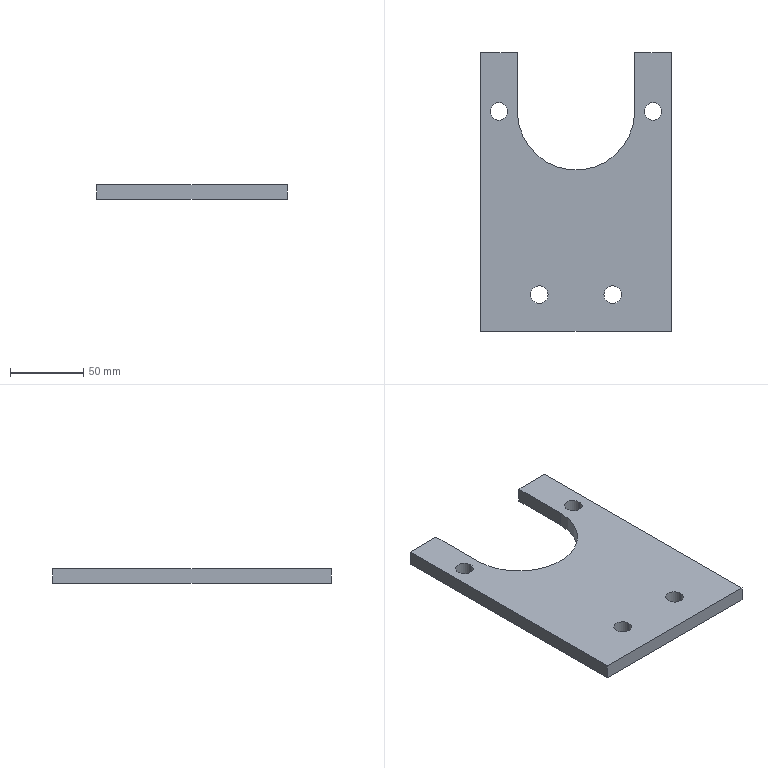Part | SolidWorks | features Extrusion 1 | 1 solid | 18 faces | box 130 x 190 x 10 mm | volume 185343 mm3 | cylinder 9 | plane 9 | commonest cylinder face diameters 12 x8 80 x1
STEP:
#1=CARTESIAN_POINT('',(84.,25.,10.));
#2=VERTEX_POINT('',#1);
#3=CARTESIAN_POINT('',(96.,25.,10.));
#4=VERTEX_POINT('',#3);
#5=CARTESIAN_POINT('',(90.,25.,10.));
#6=DIRECTION('',(0.,0.,1.));
#7=DIRECTION('',(1.,0.,0.));
#8=AXIS2_PLACEMENT_3D('',#5,#6,#7);
#9=CIRCLE('',#8,6.);
#10=EDGE_CURVE('',#2,#4,#9,.T.);
#11=ORIENTED_EDGE('',*,*,#10,.T.);
#12=CARTESIAN_POINT('',(96.,25.,0.));
#13=VERTEX_POINT('',#12);
#14=CARTESIAN_POINT('',(96.,25.,10.));
#15=DIRECTION('',(0.,0.,-1.));
#16=VECTOR('',#15,1000.);
#17=LINE('',#14,#16);
#18=EDGE_CURVE('',#4,#13,#17,.T.);
#19=ORIENTED_EDGE('',*,*,#18,.T.);
#20=CARTESIAN_POINT('',(84.,25.,0.));
#21=VERTEX_POINT('',#20);
#22=CARTESIAN_POINT('',(90.,25.,0.));
#23=DIRECTION('',(0.,0.,1.));
#24=DIRECTION('',(1.,0.,0.));
#25=AXIS2_PLACEMENT_3D('',#22,#23,#24);
#26=CIRCLE('',#25,6.);
#27=EDGE_CURVE('',#21,#13,#26,.T.);
#28=ORIENTED_EDGE('',*,*,#27,.F.);
#29=CARTESIAN_POINT('',(84.,25.,10.));
#30=DIRECTION('',(0.,0.,-1.));
#31=VECTOR('',#30,1000.);
#32=LINE('',#29,#31);
#33=EDGE_CURVE('',#2,#21,#32,.T.);
#34=ORIENTED_EDGE('',*,*,#33,.F.);
#35=EDGE_LOOP('',(#11,#19,#28,#34));
#36=FACE_OUTER_BOUND('',#35,.T.);
#37=CARTESIAN_POINT('',(90.,25.,10.));
#38=DIRECTION('',(0.,0.,-1.));
#39=DIRECTION('',(-1.,0.,0.));
#40=AXIS2_PLACEMENT_3D('',#37,#38,#39);
#41=CYLINDRICAL_SURFACE('',#40,6.);
#42=ADVANCED_FACE('',(#36),#41,.F.);
#43=CARTESIAN_POINT('',(34.,25.,10.));
#44=VERTEX_POINT('',#43);
#45=CARTESIAN_POINT('',(46.,25.,10.));
#46=VERTEX_POINT('',#45);
#47=CARTESIAN_POINT('',(40.,25.,10.));
#48=DIRECTION('',(0.,0.,1.));
#49=DIRECTION('',(1.,0.,0.));
#50=AXIS2_PLACEMENT_3D('',#47,#48,#49);
#51=CIRCLE('',#50,6.);
#52=EDGE_CURVE('',#44,#46,#51,.T.);
#53=ORIENTED_EDGE('',*,*,#52,.T.);
#54=CARTESIAN_POINT('',(46.,25.,0.));
#55=VERTEX_POINT('',#54);
#56=CARTESIAN_POINT('',(46.,25.,10.));
#57=DIRECTION('',(0.,0.,-1.));
#58=VECTOR('',#57,1000.);
#59=LINE('',#56,#58);
#60=EDGE_CURVE('',#46,#55,#59,.T.);
#61=ORIENTED_EDGE('',*,*,#60,.T.);
#62=CARTESIAN_POINT('',(34.,25.,0.));
#63=VERTEX_POINT('',#62);
#64=CARTESIAN_POINT('',(40.,25.,0.));
#65=DIRECTION('',(0.,0.,1.));
#66=DIRECTION('',(1.,0.,0.));
#67=AXIS2_PLACEMENT_3D('',#64,#65,#66);
#68=CIRCLE('',#67,6.);
#69=EDGE_CURVE('',#63,#55,#68,.T.);
#70=ORIENTED_EDGE('',*,*,#69,.F.);
#71=CARTESIAN_POINT('',(34.,25.,10.));
#72=DIRECTION('',(0.,0.,-1.));
#73=VECTOR('',#72,1000.);
#74=LINE('',#71,#73);
#75=EDGE_CURVE('',#44,#63,#74,.T.);
#76=ORIENTED_EDGE('',*,*,#75,.F.);
#77=EDGE_LOOP('',(#53,#61,#70,#76));
#78=FACE_OUTER_BOUND('',#77,.T.);
#79=CARTESIAN_POINT('',(40.,25.,10.));
#80=DIRECTION('',(0.,0.,-1.));
#81=DIRECTION('',(-1.,0.,0.));
#82=AXIS2_PLACEMENT_3D('',#79,#80,#81);
#83=CYLINDRICAL_SURFACE('',#82,6.);
#84=ADVANCED_FACE('',(#78),#83,.F.);
#85=CARTESIAN_POINT('',(6.5,150.,10.));
#86=VERTEX_POINT('',#85);
#87=CARTESIAN_POINT('',(18.5,150.,10.));
#88=VERTEX_POINT('',#87);
#89=CARTESIAN_POINT('',(12.5,150.,10.));
#90=DIRECTION('',(0.,0.,1.));
#91=DIRECTION('',(1.,0.,0.));
#92=AXIS2_PLACEMENT_3D('',#89,#90,#91);
#93=CIRCLE('',#92,6.);
#94=EDGE_CURVE('',#86,#88,#93,.T.);
#95=ORIENTED_EDGE('',*,*,#94,.T.);
#96=CARTESIAN_POINT('',(18.5,150.,0.));
#97=VERTEX_POINT('',#96);
#98=CARTESIAN_POINT('',(18.5,150.,10.));
#99=DIRECTION('',(0.,0.,-1.));
#100=VECTOR('',#99,1000.);
#101=LINE('',#98,#100);
#102=EDGE_CURVE('',#88,#97,#101,.T.);
#103=ORIENTED_EDGE('',*,*,#102,.T.);
#104=CARTESIAN_POINT('',(6.5,150.,0.));
#105=VERTEX_POINT('',#104);
#106=CARTESIAN_POINT('',(12.5,150.,0.));
#107=DIRECTION('',(0.,0.,1.));
#108=DIRECTION('',(1.,0.,0.));
#109=AXIS2_PLACEMENT_3D('',#106,#107,#108);
#110=CIRCLE('',#109,6.);
#111=EDGE_CURVE('',#105,#97,#110,.T.);
#112=ORIENTED_EDGE('',*,*,#111,.F.);
#113=CARTESIAN_POINT('',(6.5,150.,10.));
#114=DIRECTION('',(0.,0.,-1.));
#115=VECTOR('',#114,1000.);
#116=LINE('',#113,#115);
#117=EDGE_CURVE('',#86,#105,#116,.T.);
#118=ORIENTED_EDGE('',*,*,#117,.F.);
#119=EDGE_LOOP('',(#95,#103,#112,#118));
#120=FACE_OUTER_BOUND('',#119,.T.);
#121=CARTESIAN_POINT('',(12.5,150.,10.));
#122=DIRECTION('',(0.,0.,-1.));
#123=DIRECTION('',(-1.,0.,0.));
#124=AXIS2_PLACEMENT_3D('',#121,#122,#123);
#125=CYLINDRICAL_SURFACE('',#124,6.);
#126=ADVANCED_FACE('',(#120),#125,.F.);
#127=CARTESIAN_POINT('',(111.5,150.,10.));
#128=VERTEX_POINT('',#127);
#129=CARTESIAN_POINT('',(123.5,150.,10.));
#130=VERTEX_POINT('',#129);
#131=CARTESIAN_POINT('',(117.5,150.,10.));
#132=DIRECTION('',(0.,0.,1.));
#133=DIRECTION('',(1.,0.,0.));
#134=AXIS2_PLACEMENT_3D('',#131,#132,#133);
#135=CIRCLE('',#134,6.);
#136=EDGE_CURVE('',#128,#130,#135,.T.);
#137=ORIENTED_EDGE('',*,*,#136,.T.);
#138=CARTESIAN_POINT('',(123.5,150.,0.));
#139=VERTEX_POINT('',#138);
#140=CARTESIAN_POINT('',(123.5,150.,10.));
#141=DIRECTION('',(0.,0.,-1.));
#142=VECTOR('',#141,1000.);
#143=LINE('',#140,#142);
#144=EDGE_CURVE('',#130,#139,#143,.T.);
#145=ORIENTED_EDGE('',*,*,#144,.T.);
#146=CARTESIAN_POINT('',(111.5,150.,0.));
#147=VERTEX_POINT('',#146);
#148=CARTESIAN_POINT('',(117.5,150.,0.));
#149=DIRECTION('',(0.,0.,1.));
#150=DIRECTION('',(1.,0.,0.));
#151=AXIS2_PLACEMENT_3D('',#148,#149,#150);
#152=CIRCLE('',#151,6.);
#153=EDGE_CURVE('',#147,#139,#152,.T.);
#154=ORIENTED_EDGE('',*,*,#153,.F.);
#155=CARTESIAN_POINT('',(111.5,150.,10.));
#156=DIRECTION('',(0.,0.,-1.));
#157=VECTOR('',#156,1000.);
#158=LINE('',#155,#157);
#159=EDGE_CURVE('',#128,#147,#158,.T.);
#160=ORIENTED_EDGE('',*,*,#159,.F.);
#161=EDGE_LOOP('',(#137,#145,#154,#160));
#162=FACE_OUTER_BOUND('',#161,.T.);
#163=CARTESIAN_POINT('',(117.5,150.,10.));
#164=DIRECTION('',(0.,0.,-1.));
#165=DIRECTION('',(-1.,0.,0.));
#166=AXIS2_PLACEMENT_3D('',#163,#164,#165);
#167=CYLINDRICAL_SURFACE('',#166,6.);
#168=ADVANCED_FACE('',(#162),#167,.F.);
#169=ORIENTED_EDGE('',*,*,#52,.F.);
#170=CARTESIAN_POINT('',(40.,25.,10.));
#171=DIRECTION('',(0.,0.,1.));
#172=DIRECTION('',(1.,0.,0.));
#173=AXIS2_PLACEMENT_3D('',#170,#171,#172);
#174=CIRCLE('',#173,6.);
#175=EDGE_CURVE('',#46,#44,#174,.T.);
#176=ORIENTED_EDGE('',*,*,#175,.F.);
#177=EDGE_LOOP('',(#169,#176));
#178=FACE_BOUND('',#177,.T.);
#179=ORIENTED_EDGE('',*,*,#136,.F.);
#180=CARTESIAN_POINT('',(117.5,150.,10.));
#181=DIRECTION('',(0.,0.,1.));
#182=DIRECTION('',(1.,0.,0.));
#183=AXIS2_PLACEMENT_3D('',#180,#181,#182);
#184=CIRCLE('',#183,6.);
#185=EDGE_CURVE('',#130,#128,#184,.T.);
#186=ORIENTED_EDGE('',*,*,#185,.F.);
#187=EDGE_LOOP('',(#179,#186));
#188=FACE_BOUND('',#187,.T.);
#189=CARTESIAN_POINT('',(0.,190.,10.));
#190=VERTEX_POINT('',#189);
#191=CARTESIAN_POINT('',(0.,0.,10.));
#192=VERTEX_POINT('',#191);
#193=CARTESIAN_POINT('',(0.,190.,10.));
#194=DIRECTION('',(0.,-1.,0.));
#195=VECTOR('',#194,1000.);
#196=LINE('',#193,#195);
#197=EDGE_CURVE('',#190,#192,#196,.T.);
#198=ORIENTED_EDGE('',*,*,#197,.T.);
#199=CARTESIAN_POINT('',(130.,0.,10.));
#200=VERTEX_POINT('',#199);
#201=CARTESIAN_POINT('',(0.,0.,10.));
#202=DIRECTION('',(1.,0.,0.));
#203=VECTOR('',#202,1000.);
#204=LINE('',#201,#203);
#205=EDGE_CURVE('',#192,#200,#204,.T.);
#206=ORIENTED_EDGE('',*,*,#205,.T.);
#207=CARTESIAN_POINT('',(130.,190.,10.));
#208=VERTEX_POINT('',#207);
#209=CARTESIAN_POINT('',(130.,0.,10.));
#210=DIRECTION('',(0.,1.,0.));
#211=VECTOR('',#210,1000.);
#212=LINE('',#209,#211);
#213=EDGE_CURVE('',#200,#208,#212,.T.);
#214=ORIENTED_EDGE('',*,*,#213,.T.);
#215=CARTESIAN_POINT('',(105.,190.,10.));
#216=VERTEX_POINT('',#215);
#217=CARTESIAN_POINT('',(130.,190.,10.));
#218=DIRECTION('',(-1.,0.,0.));
#219=VECTOR('',#218,1000.);
#220=LINE('',#217,#219);
#221=EDGE_CURVE('',#208,#216,#220,.T.);
#222=ORIENTED_EDGE('',*,*,#221,.T.);
#223=CARTESIAN_POINT('',(105.,150.,10.));
#224=VERTEX_POINT('',#223);
#225=CARTESIAN_POINT('',(105.,190.,10.));
#226=DIRECTION('',(0.,-1.,0.));
#227=VECTOR('',#226,1000.);
#228=LINE('',#225,#227);
#229=EDGE_CURVE('',#216,#224,#228,.T.);
#230=ORIENTED_EDGE('',*,*,#229,.T.);
#231=CARTESIAN_POINT('',(25.,150.,10.));
#232=VERTEX_POINT('',#231);
#233=CARTESIAN_POINT('',(65.,150.,10.));
#234=DIRECTION('',(0.,0.,-1.));
#235=DIRECTION('',(1.,0.,0.));
#236=AXIS2_PLACEMENT_3D('',#233,#234,#235);
#237=CIRCLE('',#236,40.);
#238=EDGE_CURVE('',#224,#232,#237,.T.);
#239=ORIENTED_EDGE('',*,*,#238,.T.);
#240=CARTESIAN_POINT('',(25.,190.,10.));
#241=VERTEX_POINT('',#240);
#242=CARTESIAN_POINT('',(25.,150.,10.));
#243=DIRECTION('',(0.,1.,0.));
#244=VECTOR('',#243,1000.);
#245=LINE('',#242,#244);
#246=EDGE_CURVE('',#232,#241,#245,.T.);
#247=ORIENTED_EDGE('',*,*,#246,.T.);
#248=CARTESIAN_POINT('',(25.,190.,10.));
#249=DIRECTION('',(-1.,0.,0.));
#250=VECTOR('',#249,1000.);
#251=LINE('',#248,#250);
#252=EDGE_CURVE('',#241,#190,#251,.T.);
#253=ORIENTED_EDGE('',*,*,#252,.T.);
#254=EDGE_LOOP('',(#198,#206,#214,#222,#230,#239,#247,#253));
#255=FACE_OUTER_BOUND('',#254,.T.);
#256=ORIENTED_EDGE('',*,*,#94,.F.);
#257=CARTESIAN_POINT('',(12.5,150.,10.));
#258=DIRECTION('',(0.,0.,1.));
#259=DIRECTION('',(1.,0.,0.));
#260=AXIS2_PLACEMENT_3D('',#257,#258,#259);
#261=CIRCLE('',#260,6.);
#262=EDGE_CURVE('',#88,#86,#261,.T.);
#263=ORIENTED_EDGE('',*,*,#262,.F.);
#264=EDGE_LOOP('',(#256,#263));
#265=FACE_BOUND('',#264,.T.);
#266=ORIENTED_EDGE('',*,*,#10,.F.);
#267=CARTESIAN_POINT('',(90.,25.,10.));
#268=DIRECTION('',(0.,0.,1.));
#269=DIRECTION('',(1.,0.,0.));
#270=AXIS2_PLACEMENT_3D('',#267,#268,#269);
#271=CIRCLE('',#270,6.);
#272=EDGE_CURVE('',#4,#2,#271,.T.);
#273=ORIENTED_EDGE('',*,*,#272,.F.);
#274=EDGE_LOOP('',(#266,#273));
#275=FACE_BOUND('',#274,.T.);
#276=CARTESIAN_POINT('',(65.,150.,10.));
#277=DIRECTION('',(0.,0.,1.));
#278=DIRECTION('',(1.,0.,0.));
#279=AXIS2_PLACEMENT_3D('',#276,#277,#278);
#280=PLANE('',#279);
#281=ADVANCED_FACE('',(#178,#188,#255,#265,#275),#280,.T.);
#282=ORIENTED_EDGE('',*,*,#69,.T.);
#283=CARTESIAN_POINT('',(40.,25.,0.));
#284=DIRECTION('',(0.,0.,1.));
#285=DIRECTION('',(1.,0.,0.));
#286=AXIS2_PLACEMENT_3D('',#283,#284,#285);
#287=CIRCLE('',#286,6.);
#288=EDGE_CURVE('',#55,#63,#287,.T.);
#289=ORIENTED_EDGE('',*,*,#288,.T.);
#290=EDGE_LOOP('',(#282,#289));
#291=FACE_BOUND('',#290,.T.);
#292=ORIENTED_EDGE('',*,*,#153,.T.);
#293=CARTESIAN_POINT('',(117.5,150.,0.));
#294=DIRECTION('',(0.,0.,1.));
#295=DIRECTION('',(1.,0.,0.));
#296=AXIS2_PLACEMENT_3D('',#293,#294,#295);
#297=CIRCLE('',#296,6.);
#298=EDGE_CURVE('',#139,#147,#297,.T.);
#299=ORIENTED_EDGE('',*,*,#298,.T.);
#300=EDGE_LOOP('',(#292,#299));
#301=FACE_BOUND('',#300,.T.);
#302=CARTESIAN_POINT('',(0.,190.,0.));
#303=VERTEX_POINT('',#302);
#304=CARTESIAN_POINT('',(0.,0.,0.));
#305=VERTEX_POINT('',#304);
#306=CARTESIAN_POINT('',(0.,190.,0.));
#307=DIRECTION('',(0.,-1.,0.));
#308=VECTOR('',#307,1000.);
#309=LINE('',#306,#308);
#310=EDGE_CURVE('',#303,#305,#309,.T.);
#311=ORIENTED_EDGE('',*,*,#310,.F.);
#312=CARTESIAN_POINT('',(25.,190.,0.));
#313=VERTEX_POINT('',#312);
#314=CARTESIAN_POINT('',(25.,190.,0.));
#315=DIRECTION('',(-1.,0.,0.));
#316=VECTOR('',#315,1000.);
#317=LINE('',#314,#316);
#318=EDGE_CURVE('',#313,#303,#317,.T.);
#319=ORIENTED_EDGE('',*,*,#318,.F.);
#320=CARTESIAN_POINT('',(25.,150.,0.));
#321=VERTEX_POINT('',#320);
#322=CARTESIAN_POINT('',(25.,150.,0.));
#323=DIRECTION('',(0.,1.,0.));
#324=VECTOR('',#323,1000.);
#325=LINE('',#322,#324);
#326=EDGE_CURVE('',#321,#313,#325,.T.);
#327=ORIENTED_EDGE('',*,*,#326,.F.);
#328=CARTESIAN_POINT('',(105.,150.,0.));
#329=VERTEX_POINT('',#328);
#330=CARTESIAN_POINT('',(65.,150.,0.));
#331=DIRECTION('',(0.,0.,-1.));
#332=DIRECTION('',(1.,0.,0.));
#333=AXIS2_PLACEMENT_3D('',#330,#331,#332);
#334=CIRCLE('',#333,40.);
#335=EDGE_CURVE('',#329,#321,#334,.T.);
#336=ORIENTED_EDGE('',*,*,#335,.F.);
#337=CARTESIAN_POINT('',(105.,190.,0.));
#338=VERTEX_POINT('',#337);
#339=CARTESIAN_POINT('',(105.,190.,0.));
#340=DIRECTION('',(0.,-1.,0.));
#341=VECTOR('',#340,1000.);
#342=LINE('',#339,#341);
#343=EDGE_CURVE('',#338,#329,#342,.T.);
#344=ORIENTED_EDGE('',*,*,#343,.F.);
#345=CARTESIAN_POINT('',(130.,190.,0.));
#346=VERTEX_POINT('',#345);
#347=CARTESIAN_POINT('',(130.,190.,0.));
#348=DIRECTION('',(-1.,0.,0.));
#349=VECTOR('',#348,1000.);
#350=LINE('',#347,#349);
#351=EDGE_CURVE('',#346,#338,#350,.T.);
#352=ORIENTED_EDGE('',*,*,#351,.F.);
#353=CARTESIAN_POINT('',(130.,0.,0.));
#354=VERTEX_POINT('',#353);
#355=CARTESIAN_POINT('',(130.,0.,0.));
#356=DIRECTION('',(0.,1.,0.));
#357=VECTOR('',#356,1000.);
#358=LINE('',#355,#357);
#359=EDGE_CURVE('',#354,#346,#358,.T.);
#360=ORIENTED_EDGE('',*,*,#359,.F.);
#361=CARTESIAN_POINT('',(0.,0.,0.));
#362=DIRECTION('',(1.,0.,0.));
#363=VECTOR('',#362,1000.);
#364=LINE('',#361,#363);
#365=EDGE_CURVE('',#305,#354,#364,.T.);
#366=ORIENTED_EDGE('',*,*,#365,.F.);
#367=EDGE_LOOP('',(#311,#319,#327,#336,#344,#352,#360,#366));
#368=FACE_OUTER_BOUND('',#367,.T.);
#369=ORIENTED_EDGE('',*,*,#111,.T.);
#370=CARTESIAN_POINT('',(12.5,150.,0.));
#371=DIRECTION('',(0.,0.,1.));
#372=DIRECTION('',(1.,0.,0.));
#373=AXIS2_PLACEMENT_3D('',#370,#371,#372);
#374=CIRCLE('',#373,6.);
#375=EDGE_CURVE('',#97,#105,#374,.T.);
#376=ORIENTED_EDGE('',*,*,#375,.T.);
#377=EDGE_LOOP('',(#369,#376));
#378=FACE_BOUND('',#377,.T.);
#379=ORIENTED_EDGE('',*,*,#27,.T.);
#380=CARTESIAN_POINT('',(90.,25.,0.));
#381=DIRECTION('',(0.,0.,1.));
#382=DIRECTION('',(1.,0.,0.));
#383=AXIS2_PLACEMENT_3D('',#380,#381,#382);
#384=CIRCLE('',#383,6.);
#385=EDGE_CURVE('',#13,#21,#384,.T.);
#386=ORIENTED_EDGE('',*,*,#385,.T.);
#387=EDGE_LOOP('',(#379,#386));
#388=FACE_BOUND('',#387,.T.);
#389=CARTESIAN_POINT('',(65.,150.,0.));
#390=DIRECTION('',(0.,0.,1.));
#391=DIRECTION('',(1.,0.,0.));
#392=AXIS2_PLACEMENT_3D('',#389,#390,#391);
#393=PLANE('',#392);
#394=ADVANCED_FACE('',(#291,#301,#368,#378,#388),#393,.F.);
#395=ORIENTED_EDGE('',*,*,#310,.T.);
#396=CARTESIAN_POINT('',(0.,0.,10.));
#397=DIRECTION('',(0.,0.,-1.));
#398=VECTOR('',#397,1000.);
#399=LINE('',#396,#398);
#400=EDGE_CURVE('',#192,#305,#399,.T.);
#401=ORIENTED_EDGE('',*,*,#400,.F.);
#402=ORIENTED_EDGE('',*,*,#197,.F.);
#403=CARTESIAN_POINT('',(0.,190.,10.));
#404=DIRECTION('',(0.,0.,-1.));
#405=VECTOR('',#404,1000.);
#406=LINE('',#403,#405);
#407=EDGE_CURVE('',#190,#303,#406,.T.);
#408=ORIENTED_EDGE('',*,*,#407,.T.);
#409=EDGE_LOOP('',(#395,#401,#402,#408));
#410=FACE_OUTER_BOUND('',#409,.T.);
#411=CARTESIAN_POINT('',(0.,190.,10.));
#412=DIRECTION('',(1.,0.,0.));
#413=DIRECTION('',(0.,1.,0.));
#414=AXIS2_PLACEMENT_3D('',#411,#412,#413);
#415=PLANE('',#414);
#416=ADVANCED_FACE('',(#410),#415,.F.);
#417=ORIENTED_EDGE('',*,*,#365,.T.);
#418=CARTESIAN_POINT('',(130.,0.,10.));
#419=DIRECTION('',(0.,0.,-1.));
#420=VECTOR('',#419,1000.);
#421=LINE('',#418,#420);
#422=EDGE_CURVE('',#200,#354,#421,.T.);
#423=ORIENTED_EDGE('',*,*,#422,.F.);
#424=ORIENTED_EDGE('',*,*,#205,.F.);
#425=ORIENTED_EDGE('',*,*,#400,.T.);
#426=EDGE_LOOP('',(#417,#423,#424,#425));
#427=FACE_OUTER_BOUND('',#426,.T.);
#428=CARTESIAN_POINT('',(0.,0.,10.));
#429=DIRECTION('',(0.,1.,0.));
#430=DIRECTION('',(0.,0.,1.));
#431=AXIS2_PLACEMENT_3D('',#428,#429,#430);
#432=PLANE('',#431);
#433=ADVANCED_FACE('',(#427),#432,.F.);
#434=ORIENTED_EDGE('',*,*,#359,.T.);
#435=CARTESIAN_POINT('',(130.,190.,10.));
#436=DIRECTION('',(0.,0.,-1.));
#437=VECTOR('',#436,1000.);
#438=LINE('',#435,#437);
#439=EDGE_CURVE('',#208,#346,#438,.T.);
#440=ORIENTED_EDGE('',*,*,#439,.F.);
#441=ORIENTED_EDGE('',*,*,#213,.F.);
#442=ORIENTED_EDGE('',*,*,#422,.T.);
#443=EDGE_LOOP('',(#434,#440,#441,#442));
#444=FACE_OUTER_BOUND('',#443,.T.);
#445=CARTESIAN_POINT('',(130.,0.,10.));
#446=DIRECTION('',(-1.,0.,0.));
#447=DIRECTION('',(0.,0.,1.));
#448=AXIS2_PLACEMENT_3D('',#445,#446,#447);
#449=PLANE('',#448);
#450=ADVANCED_FACE('',(#444),#449,.F.);
#451=ORIENTED_EDGE('',*,*,#351,.T.);
#452=CARTESIAN_POINT('',(105.,190.,10.));
#453=DIRECTION('',(0.,0.,-1.));
#454=VECTOR('',#453,1000.);
#455=LINE('',#452,#454);
#456=EDGE_CURVE('',#216,#338,#455,.T.);
#457=ORIENTED_EDGE('',*,*,#456,.F.);
#458=ORIENTED_EDGE('',*,*,#221,.F.);
#459=ORIENTED_EDGE('',*,*,#439,.T.);
#460=EDGE_LOOP('',(#451,#457,#458,#459));
#461=FACE_OUTER_BOUND('',#460,.T.);
#462=CARTESIAN_POINT('',(130.,190.,10.));
#463=DIRECTION('',(0.,-1.,0.));
#464=DIRECTION('',(0.,0.,-1.));
#465=AXIS2_PLACEMENT_3D('',#462,#463,#464);
#466=PLANE('',#465);
#467=ADVANCED_FACE('',(#461),#466,.F.);
#468=ORIENTED_EDGE('',*,*,#343,.T.);
#469=CARTESIAN_POINT('',(105.,150.,10.));
#470=DIRECTION('',(0.,0.,-1.));
#471=VECTOR('',#470,1000.);
#472=LINE('',#469,#471);
#473=EDGE_CURVE('',#224,#329,#472,.T.);
#474=ORIENTED_EDGE('',*,*,#473,.F.);
#475=ORIENTED_EDGE('',*,*,#229,.F.);
#476=ORIENTED_EDGE('',*,*,#456,.T.);
#477=EDGE_LOOP('',(#468,#474,#475,#476));
#478=FACE_OUTER_BOUND('',#477,.T.);
#479=CARTESIAN_POINT('',(105.,190.,10.));
#480=DIRECTION('',(1.,0.,0.));
#481=DIRECTION('',(0.,0.,-1.));
#482=AXIS2_PLACEMENT_3D('',#479,#480,#481);
#483=PLANE('',#482);
#484=ADVANCED_FACE('',(#478),#483,.F.);
#485=ORIENTED_EDGE('',*,*,#335,.T.);
#486=CARTESIAN_POINT('',(25.,150.,10.));
#487=DIRECTION('',(0.,0.,-1.));
#488=VECTOR('',#487,1000.);
#489=LINE('',#486,#488);
#490=EDGE_CURVE('',#232,#321,#489,.T.);
#491=ORIENTED_EDGE('',*,*,#490,.F.);
#492=ORIENTED_EDGE('',*,*,#238,.F.);
#493=ORIENTED_EDGE('',*,*,#473,.T.);
#494=EDGE_LOOP('',(#485,#491,#492,#493));
#495=FACE_OUTER_BOUND('',#494,.T.);
#496=CARTESIAN_POINT('',(65.,150.,10.));
#497=DIRECTION('',(0.,0.,-1.));
#498=DIRECTION('',(-1.,0.,0.));
#499=AXIS2_PLACEMENT_3D('',#496,#497,#498);
#500=CYLINDRICAL_SURFACE('',#499,40.);
#501=ADVANCED_FACE('',(#495),#500,.F.);
#502=ORIENTED_EDGE('',*,*,#326,.T.);
#503=CARTESIAN_POINT('',(25.,190.,10.));
#504=DIRECTION('',(0.,0.,-1.));
#505=VECTOR('',#504,1000.);
#506=LINE('',#503,#505);
#507=EDGE_CURVE('',#241,#313,#506,.T.);
#508=ORIENTED_EDGE('',*,*,#507,.F.);
#509=ORIENTED_EDGE('',*,*,#246,.F.);
#510=ORIENTED_EDGE('',*,*,#490,.T.);
#511=EDGE_LOOP('',(#502,#508,#509,#510));
#512=FACE_OUTER_BOUND('',#511,.T.);
#513=CARTESIAN_POINT('',(25.,150.,10.));
#514=DIRECTION('',(-1.,0.,0.));
#515=DIRECTION('',(0.,0.,1.));
#516=AXIS2_PLACEMENT_3D('',#513,#514,#515);
#517=PLANE('',#516);
#518=ADVANCED_FACE('',(#512),#517,.F.);
#519=ORIENTED_EDGE('',*,*,#318,.T.);
#520=ORIENTED_EDGE('',*,*,#407,.F.);
#521=ORIENTED_EDGE('',*,*,#252,.F.);
#522=ORIENTED_EDGE('',*,*,#507,.T.);
#523=EDGE_LOOP('',(#519,#520,#521,#522));
#524=FACE_OUTER_BOUND('',#523,.T.);
#525=CARTESIAN_POINT('',(25.,190.,10.));
#526=DIRECTION('',(0.,-1.,0.));
#527=DIRECTION('',(0.,0.,-1.));
#528=AXIS2_PLACEMENT_3D('',#525,#526,#527);
#529=PLANE('',#528);
#530=ADVANCED_FACE('',(#524),#529,.F.);
#531=ORIENTED_EDGE('',*,*,#144,.F.);
#532=ORIENTED_EDGE('',*,*,#185,.T.);
#533=ORIENTED_EDGE('',*,*,#159,.T.);
#534=ORIENTED_EDGE('',*,*,#298,.F.);
#535=EDGE_LOOP('',(#531,#532,#533,#534));
#536=FACE_OUTER_BOUND('',#535,.T.);
#537=CARTESIAN_POINT('',(117.5,150.,10.));
#538=DIRECTION('',(0.,0.,-1.));
#539=DIRECTION('',(-1.,0.,0.));
#540=AXIS2_PLACEMENT_3D('',#537,#538,#539);
#541=CYLINDRICAL_SURFACE('',#540,6.);
#542=ADVANCED_FACE('',(#536),#541,.F.);
#543=ORIENTED_EDGE('',*,*,#102,.F.);
#544=ORIENTED_EDGE('',*,*,#262,.T.);
#545=ORIENTED_EDGE('',*,*,#117,.T.);
#546=ORIENTED_EDGE('',*,*,#375,.F.);
#547=EDGE_LOOP('',(#543,#544,#545,#546));
#548=FACE_OUTER_BOUND('',#547,.T.);
#549=CARTESIAN_POINT('',(12.5,150.,10.));
#550=DIRECTION('',(0.,0.,-1.));
#551=DIRECTION('',(-1.,0.,0.));
#552=AXIS2_PLACEMENT_3D('',#549,#550,#551);
#553=CYLINDRICAL_SURFACE('',#552,6.);
#554=ADVANCED_FACE('',(#548),#553,.F.);
#555=ORIENTED_EDGE('',*,*,#60,.F.);
#556=ORIENTED_EDGE('',*,*,#175,.T.);
#557=ORIENTED_EDGE('',*,*,#75,.T.);
#558=ORIENTED_EDGE('',*,*,#288,.F.);
#559=EDGE_LOOP('',(#555,#556,#557,#558));
#560=FACE_OUTER_BOUND('',#559,.T.);
#561=CARTESIAN_POINT('',(40.,25.,10.));
#562=DIRECTION('',(0.,0.,-1.));
#563=DIRECTION('',(-1.,0.,0.));
#564=AXIS2_PLACEMENT_3D('',#561,#562,#563);
#565=CYLINDRICAL_SURFACE('',#564,6.);
#566=ADVANCED_FACE('',(#560),#565,.F.);
#567=ORIENTED_EDGE('',*,*,#18,.F.);
#568=ORIENTED_EDGE('',*,*,#272,.T.);
#569=ORIENTED_EDGE('',*,*,#33,.T.);
#570=ORIENTED_EDGE('',*,*,#385,.F.);
#571=EDGE_LOOP('',(#567,#568,#569,#570));
#572=FACE_OUTER_BOUND('',#571,.T.);
#573=CARTESIAN_POINT('',(90.,25.,10.));
#574=DIRECTION('',(0.,0.,-1.));
#575=DIRECTION('',(-1.,0.,0.));
#576=AXIS2_PLACEMENT_3D('',#573,#574,#575);
#577=CYLINDRICAL_SURFACE('',#576,6.);
#578=ADVANCED_FACE('',(#572),#577,.F.);
#579=CLOSED_SHELL('',(#42,#84,#126,#168,#281,#394,#416,#433,#450,#467,#484,#501,#518,#530,#542,#554,#566,#578));
#580=MANIFOLD_SOLID_BREP('',#579);
#581=CARTESIAN_POINT('',(0.,0.,0.));
#582=DIRECTION('',(0.,0.,1.));
#583=DIRECTION('',(1.,0.,0.));
#584=AXIS2_PLACEMENT_3D('',#581,#582,#583);
#585=(LENGTH_UNIT()NAMED_UNIT(*)SI_UNIT(.MILLI.,.METRE.));
#586=UNCERTAINTY_MEASURE_WITH_UNIT(LENGTH_MEASURE(0.00001),#585,'','');
#587=(NAMED_UNIT(*)PLANE_ANGLE_UNIT()SI_UNIT($,.RADIAN.));
#588=(NAMED_UNIT(*)SI_UNIT($,.STERADIAN.)SOLID_ANGLE_UNIT());
#589=(GEOMETRIC_REPRESENTATION_CONTEXT(3)GLOBAL_UNCERTAINTY_ASSIGNED_CONTEXT((#586))GLOBAL_UNIT_ASSIGNED_CONTEXT((#585,#587,#588))REPRESENTATION_CONTEXT('',''));
#590=ADVANCED_BREP_SHAPE_REPRESENTATION('',(#580,#584),#589);